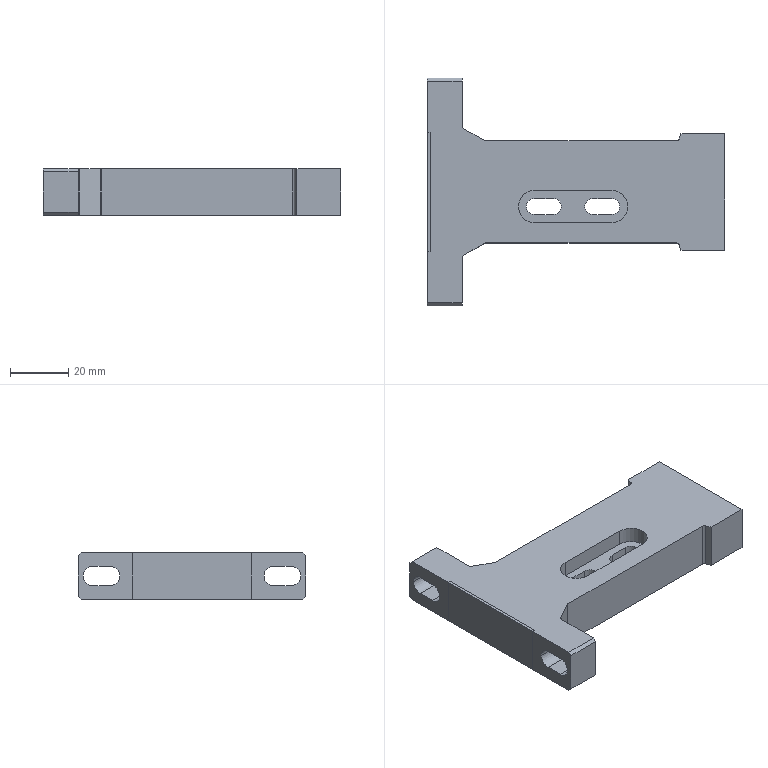NC program | NX | posted with a generic post | part box 102 x 78 x 16 mm
Lines 1 to 852 of 2996:
N10 G17 G21 G94 G90
(ZLEVEL_PROFILE_COPY_COPY_1_COPY_1_COPY_COPY , TOOL : D4)
N12 T04 M6
N14 G54
N16 G17 G0 G90 X-27.95 Y-1.3 B0. C0. S9500 M3
N18 G43 Z30. H4
N20 Z1.5
N22 G94 G1 X-27.838 Z1.494 F1400.
N24 X-27.571 Y-1.238 Z1.48
N26 X-27.322 Y-1.121 Z1.465
N28 X-27.068 Y-0.92 Z1.448
N30 X-26.814 Y-0.556 Z1.425
N32 X-26.696 Y-0.127 Z1.402
N34 X-26.729 Y0.316 Z1.379
N36 X-26.908 Y0.723 Z1.355
N38 X-27.212 Y1.047 Z1.332
N40 X-27.492 Y1.208 Z1.315
N42 X-27.838 Y1.3 Z1.296
N44 X-34.162 Z0.965
N46 X-34.574 Y1.177 Z0.942
N48 X-34.925 Y0.928 Z0.92
N50 X-35.176 Y0.578 Z0.897
N52 X-35.3 Y0.165 Z0.875
N54 Y-0.158 Z0.858
N56 X-35.178 Y-0.573 Z0.835
N58 X-34.928 Y-0.925 Z0.812
N60 X-34.576 Y-1.177 Z0.79
N62 X-34.162 Y-1.3 Z0.767
N64 X-27.838 Z0.436
N66 X-27.571 Y-1.238 Z0.421
N68 X-27.322 Y-1.121 Z0.407
N70 X-27.068 Y-0.92 Z0.39
N72 X-26.814 Y-0.556 Z0.367
N74 X-26.696 Y-0.127 Z0.343
N76 X-26.729 Y0.316 Z0.32
N78 X-26.908 Y0.723 Z0.297
N80 X-27.212 Y1.047 Z0.273
N82 X-27.492 Y1.208 Z0.256
N84 X-27.838 Y1.3 Z0.238
N86 X-34.162 Z-0.094
N88 X-34.574 Y1.177 Z-0.116
N90 X-34.925 Y0.928 Z-0.139
N92 X-35.176 Y0.578 Z-0.161
N94 X-35.3 Y0.165 Z-0.184
N96 Y-0.158 Z-0.201
N98 X-35.178 Y-0.573 Z-0.224
N100 X-34.928 Y-0.925 Z-0.246
N102 X-34.576 Y-1.177 Z-0.269
N104 X-34.162 Y-1.3 Z-0.292
N106 X-34. Z-0.3
N108 X-28.
N110 G3 X-26.7 Y0. R1.3
N112 X-28. Y1.3 R1.3
N114 G1 X-34.
N116 G3 X-35.3 Y0. R1.3
N118 X-34. Y-1.3 R1.3
N120 G1 X-28.118 Z-0.417
N122 X-27.978 Y-1.294 Z-0.419
N124 X-27.839 Y-1.284 Z-0.422
N126 X-27.686 Y-1.254 Z-0.425
N128 X-27.568 Y-1.219 Z-0.428
N130 X-27.422 Y-1.158 Z-0.431
N132 X-27.318 Y-1.098 Z-0.433
N134 X-27.179 Y-0.997 Z-0.437
N136 X-27.098 Y-0.928 Z-0.439
N138 X-26.998 Y-0.821 Z-0.442
N140 X-26.922 Y-0.712 Z-0.444
N142 X-26.832 Y-0.553 Z-0.448
N144 X-26.792 Y-0.467 Z-0.45
N146 X-26.752 Y-0.337 Z-0.453
N148 X-26.723 Y-0.197 Z-0.456
N150 X-26.702 Y-0.077 Z-0.458
N152 X-26.703 Y0.081 Z-0.461
N154 X-26.75 Y0.357 Z-0.467
N156 X-26.798 Y0.496 Z-0.47
N158 X-26.855 Y0.616 Z-0.472
N160 X-26.936 Y0.733 Z-0.475
N162 X-27.018 Y0.842 Z-0.478
N164 X-27.088 Y0.918 Z-0.48
N166 X-27.125 Y0.955 Z-0.481
N168 X-27.221 Y1.032 Z-0.483
N170 X-27.368 Y1.127 Z-0.487
N172 X-27.459 Y1.176 Z-0.489
N174 X-27.596 Y1.229 Z-0.492
N176 X-27.724 Y1.262 Z-0.494
N178 X-27.861 Y1.286 Z-0.497
N180 X-28. Y1.295 Z-0.5
N182 X-28.14 Y1.3 Z-0.503
N184 X-33.042 Z-0.6
N186 X-34.
N188 G3 X-35.3 Y0. R1.3
N190 X-34. Y-1.3 R1.3
N192 G1 X-28.118 Z-0.717
N194 X-27.978 Y-1.294 Z-0.719
N196 X-27.839 Y-1.284 Z-0.722
N198 X-27.686 Y-1.254 Z-0.725
N200 X-27.568 Y-1.219 Z-0.728
N202 X-27.422 Y-1.158 Z-0.731
N204 X-27.318 Y-1.098 Z-0.733
N206 X-27.179 Y-0.997 Z-0.737
N208 X-27.098 Y-0.928 Z-0.739
N210 X-26.998 Y-0.821 Z-0.742
N212 X-26.922 Y-0.712 Z-0.744
N214 X-26.832 Y-0.553 Z-0.748
N216 X-26.792 Y-0.467 Z-0.75
N218 X-26.752 Y-0.337 Z-0.753
N220 X-26.723 Y-0.197 Z-0.756
N222 X-26.702 Y-0.077 Z-0.758
N224 X-26.703 Y0.081 Z-0.761
N226 X-26.75 Y0.357 Z-0.767
N228 X-26.798 Y0.496 Z-0.77
N230 X-26.855 Y0.616 Z-0.772
N232 X-26.936 Y0.733 Z-0.775
N234 X-27.018 Y0.842 Z-0.778
N236 X-27.089 Y0.918 Z-0.78
N238 X-27.125 Y0.955 Z-0.781
N240 X-27.221 Y1.032 Z-0.783
N242 X-27.368 Y1.127 Z-0.787
N244 X-27.459 Y1.176 Z-0.789
N246 X-27.596 Y1.229 Z-0.792
N248 X-27.724 Y1.262 Z-0.794
N250 X-27.861 Y1.286 Z-0.797
N252 X-28. Y1.295 Z-0.8
N254 X-28.14 Y1.3 Z-0.803
N256 X-33.042 Z-0.9
N258 X-34.
N260 G3 X-35.3 Y0. R1.3
N262 X-34. Y-1.3 R1.3
N264 G1 X-28.118 Z-1.017
N266 X-27.978 Y-1.294 Z-1.019
N268 X-27.839 Y-1.284 Z-1.022
N270 X-27.686 Y-1.254 Z-1.025
N272 X-27.568 Y-1.219 Z-1.028
N274 X-27.422 Y-1.158 Z-1.031
N276 X-27.318 Y-1.098 Z-1.033
N278 X-27.179 Y-0.997 Z-1.037
N280 X-27.098 Y-0.928 Z-1.039
N282 X-26.998 Y-0.821 Z-1.042
N284 X-26.922 Y-0.712 Z-1.044
N286 X-26.832 Y-0.553 Z-1.048
N288 X-26.792 Y-0.467 Z-1.05
N290 X-26.752 Y-0.337 Z-1.053
N292 X-26.723 Y-0.197 Z-1.056
N294 X-26.702 Y-0.077 Z-1.058
N296 X-26.703 Y0.081 Z-1.061
N298 X-26.75 Y0.357 Z-1.067
N300 X-26.798 Y0.496 Z-1.07
N302 X-26.855 Y0.616 Z-1.072
N304 X-26.936 Y0.733 Z-1.075
N306 X-27.018 Y0.842 Z-1.078
N308 X-27.089 Y0.918 Z-1.08
N310 X-27.125 Y0.955 Z-1.081
N312 X-27.221 Y1.032 Z-1.083
N314 X-27.368 Y1.127 Z-1.087
N316 X-27.459 Y1.176 Z-1.089
N318 X-27.596 Y1.229 Z-1.092
N320 X-27.724 Y1.262 Z-1.094
N322 X-27.861 Y1.285 Z-1.097
N324 X-28. Y1.295 Z-1.1
N326 X-28.14 Y1.3 Z-1.103
N328 X-33.042 Z-1.2
N330 X-34.
N332 G3 X-35.3 Y0. R1.3
N334 X-34. Y-1.3 R1.3
N336 G1 X-28.118 Z-1.317
N338 X-27.978 Y-1.294 Z-1.319
N340 X-27.839 Y-1.284 Z-1.322
N342 X-27.686 Y-1.254 Z-1.325
N344 X-27.568 Y-1.219 Z-1.328
N346 X-27.422 Y-1.158 Z-1.331
N348 X-27.318 Y-1.098 Z-1.333
N350 X-27.179 Y-0.997 Z-1.337
N352 X-27.098 Y-0.928 Z-1.339
N354 X-26.998 Y-0.821 Z-1.342
N356 X-26.922 Y-0.712 Z-1.344
N358 X-26.832 Y-0.553 Z-1.348
N360 X-26.792 Y-0.467 Z-1.35
N362 X-26.752 Y-0.337 Z-1.353
N364 X-26.723 Y-0.197 Z-1.356
N366 X-26.702 Y-0.077 Z-1.358
N368 X-26.703 Y0.081 Z-1.361
N370 X-26.75 Y0.357 Z-1.367
N372 X-26.798 Y0.496 Z-1.37
N374 X-26.855 Y0.616 Z-1.372
N376 X-26.936 Y0.733 Z-1.375
N378 X-27.018 Y0.842 Z-1.378
N380 X-27.089 Y0.918 Z-1.38
N382 X-27.125 Y0.955 Z-1.381
N384 X-27.221 Y1.032 Z-1.383
N386 X-27.368 Y1.127 Z-1.387
N388 X-27.459 Y1.176 Z-1.389
N390 X-27.596 Y1.229 Z-1.392
N392 X-27.724 Y1.262 Z-1.394
N394 X-27.861 Y1.285 Z-1.397
N396 X-28. Y1.295 Z-1.4
N398 X-28.14 Y1.3 Z-1.403
N400 X-33.042 Z-1.5
N402 X-34.
N404 G3 X-35.3 Y0. R1.3
N406 X-34. Y-1.3 R1.3
N408 G1 X-28.118 Z-1.617
N410 X-27.978 Y-1.294 Z-1.619
N412 X-27.839 Y-1.284 Z-1.622
N414 X-27.686 Y-1.254 Z-1.625
N416 X-27.568 Y-1.219 Z-1.628
N418 X-27.422 Y-1.158 Z-1.631
N420 X-27.318 Y-1.098 Z-1.633
N422 X-27.179 Y-0.997 Z-1.637
N424 X-27.098 Y-0.928 Z-1.639
N426 X-26.998 Y-0.821 Z-1.642
N428 X-26.922 Y-0.712 Z-1.644
N430 X-26.832 Y-0.553 Z-1.648
N432 X-26.792 Y-0.467 Z-1.65
N434 X-26.752 Y-0.337 Z-1.653
N436 X-26.723 Y-0.197 Z-1.656
N438 X-26.702 Y-0.077 Z-1.658
N440 X-26.703 Y0.081 Z-1.661
N442 X-26.75 Y0.357 Z-1.667
N444 X-26.798 Y0.496 Z-1.67
N446 X-26.855 Y0.616 Z-1.672
N448 X-26.936 Y0.733 Z-1.675
N450 X-27.018 Y0.842 Z-1.678
N452 X-27.089 Y0.918 Z-1.68
N454 X-27.125 Y0.955 Z-1.681
N456 X-27.221 Y1.032 Z-1.683
N458 X-27.368 Y1.127 Z-1.687
N460 X-27.459 Y1.176 Z-1.689
N462 X-27.595 Y1.229 Z-1.692
N464 X-27.724 Y1.262 Z-1.694
N466 X-27.861 Y1.285 Z-1.697
N468 X-28. Y1.295 Z-1.7
N470 X-28.14 Y1.3 Z-1.703
N472 X-33.042 Z-1.8
N474 X-34.
N476 G3 X-35.3 Y0. R1.3
N478 X-34. Y-1.3 R1.3
N480 G1 X-28.118 Z-1.917
N482 X-27.978 Y-1.294 Z-1.919
N484 X-27.839 Y-1.284 Z-1.922
N486 X-27.686 Y-1.254 Z-1.925
N488 X-27.568 Y-1.219 Z-1.928
N490 X-27.422 Y-1.158 Z-1.931
N492 X-27.318 Y-1.098 Z-1.933
N494 X-27.179 Y-0.997 Z-1.937
N496 X-27.098 Y-0.928 Z-1.939
N498 X-26.999 Y-0.821 Z-1.942
N500 X-26.922 Y-0.712 Z-1.944
N502 X-26.832 Y-0.553 Z-1.948
N504 X-26.792 Y-0.467 Z-1.95
N506 X-26.752 Y-0.337 Z-1.953
N508 X-26.723 Y-0.197 Z-1.956
N510 X-26.702 Y-0.077 Z-1.958
N512 X-26.703 Y0.081 Z-1.961
N514 X-26.75 Y0.357 Z-1.967
N516 X-26.798 Y0.496 Z-1.97
N518 X-26.855 Y0.616 Z-1.972
N520 X-26.936 Y0.733 Z-1.975
N522 X-27.018 Y0.842 Z-1.978
N524 X-27.089 Y0.918 Z-1.98
N526 X-27.125 Y0.955 Z-1.981
N528 X-27.221 Y1.032 Z-1.983
N530 X-27.368 Y1.127 Z-1.987
N532 X-27.459 Y1.176 Z-1.989
N534 X-27.595 Y1.229 Z-1.992
N536 X-27.724 Y1.262 Z-1.994
N538 X-27.861 Y1.285 Z-1.997
N540 X-28. Y1.295 Z-2.
N542 X-28.14 Y1.3 Z-2.003
N544 X-33.042 Z-2.1
N546 X-34.
N548 G3 X-35.3 Y0. R1.3
N550 X-34. Y-1.3 R1.3
N552 G1 X-28.118 Z-2.217
N554 X-27.978 Y-1.294 Z-2.219
N556 X-27.839 Y-1.284 Z-2.222
N558 X-27.686 Y-1.254 Z-2.225
N560 X-27.568 Y-1.219 Z-2.228
N562 X-27.422 Y-1.158 Z-2.231
N564 X-27.318 Y-1.098 Z-2.233
N566 X-27.179 Y-0.997 Z-2.237
N568 X-27.098 Y-0.928 Z-2.239
N570 X-26.999 Y-0.821 Z-2.242
N572 X-26.922 Y-0.712 Z-2.244
N574 X-26.832 Y-0.553 Z-2.248
N576 X-26.792 Y-0.467 Z-2.25
N578 X-26.752 Y-0.337 Z-2.253
N580 X-26.723 Y-0.197 Z-2.256
N582 X-26.702 Y-0.077 Z-2.258
N584 X-26.703 Y0.081 Z-2.261
N586 X-26.75 Y0.357 Z-2.267
N588 X-26.798 Y0.496 Z-2.27
N590 X-26.855 Y0.616 Z-2.272
N592 X-26.936 Y0.733 Z-2.275
N594 X-27.018 Y0.842 Z-2.278
N596 X-27.089 Y0.918 Z-2.28
N598 X-27.125 Y0.955 Z-2.281
N600 X-27.221 Y1.032 Z-2.283
N602 X-27.368 Y1.127 Z-2.287
N604 X-27.459 Y1.176 Z-2.289
N606 X-27.595 Y1.229 Z-2.292
N608 X-27.724 Y1.262 Z-2.294
N610 X-27.861 Y1.285 Z-2.297
N612 X-28. Y1.295 Z-2.3
N614 X-28.14 Y1.3 Z-2.303
N616 X-33.042 Z-2.4
N618 X-34.
N620 G3 X-35.3 Y0. R1.3
N622 X-34. Y-1.3 R1.3
N624 G1 X-28.118 Z-2.517
N626 X-27.978 Y-1.294 Z-2.519
N628 X-27.839 Y-1.284 Z-2.522
N630 X-27.686 Y-1.254 Z-2.525
N632 X-27.568 Y-1.219 Z-2.528
N634 X-27.422 Y-1.158 Z-2.531
N636 X-27.318 Y-1.098 Z-2.533
N638 X-27.179 Y-0.997 Z-2.537
N640 X-27.098 Y-0.928 Z-2.539
N642 X-26.999 Y-0.821 Z-2.542
N644 X-26.922 Y-0.712 Z-2.544
N646 X-26.832 Y-0.553 Z-2.548
N648 X-26.792 Y-0.467 Z-2.55
N650 X-26.752 Y-0.337 Z-2.553
N652 X-26.723 Y-0.197 Z-2.556
N654 X-26.702 Y-0.077 Z-2.558
N656 X-26.703 Y0.081 Z-2.561
N658 X-26.75 Y0.357 Z-2.567
N660 X-26.798 Y0.496 Z-2.57
N662 X-26.855 Y0.616 Z-2.572
N664 X-26.936 Y0.733 Z-2.575
N666 X-27.018 Y0.842 Z-2.578
N668 X-27.089 Y0.918 Z-2.58
N670 X-27.125 Y0.955 Z-2.581
N672 X-27.221 Y1.032 Z-2.583
N674 X-27.368 Y1.127 Z-2.587
N676 X-27.459 Y1.176 Z-2.589
N678 X-27.595 Y1.229 Z-2.592
N680 X-27.724 Y1.262 Z-2.594
N682 X-27.861 Y1.285 Z-2.597
N684 X-28. Y1.295 Z-2.6
N686 X-28.14 Y1.3 Z-2.603
N688 X-33.042 Z-2.7
N690 X-34.
N692 G3 X-35.3 Y0. R1.3
N694 X-34. Y-1.3 R1.3
N696 G1 X-28.118 Z-2.817
N698 X-27.978 Y-1.294 Z-2.819
N700 X-27.839 Y-1.284 Z-2.822
N702 X-27.686 Y-1.254 Z-2.825
N704 X-27.568 Y-1.219 Z-2.828
N706 X-27.422 Y-1.158 Z-2.831
N708 X-27.318 Y-1.098 Z-2.833
N710 X-27.179 Y-0.997 Z-2.837
N712 X-27.098 Y-0.928 Z-2.839
N714 X-26.999 Y-0.821 Z-2.842
N716 X-26.922 Y-0.712 Z-2.844
N718 X-26.832 Y-0.553 Z-2.848
N720 X-26.792 Y-0.467 Z-2.85
N722 X-26.752 Y-0.337 Z-2.853
N724 X-26.723 Y-0.197 Z-2.856
N726 X-26.702 Y-0.077 Z-2.858
N728 X-26.703 Y0.081 Z-2.861
N730 X-26.75 Y0.357 Z-2.867
N732 X-26.798 Y0.496 Z-2.87
N734 X-26.855 Y0.616 Z-2.872
N736 X-26.936 Y0.733 Z-2.875
N738 X-27.018 Y0.842 Z-2.878
N740 X-27.089 Y0.918 Z-2.88
N742 X-27.125 Y0.955 Z-2.881
N744 X-27.221 Y1.032 Z-2.883
N746 X-27.368 Y1.127 Z-2.887
N748 X-27.459 Y1.176 Z-2.889
N750 X-27.595 Y1.229 Z-2.892
N752 X-27.724 Y1.262 Z-2.894
N754 X-27.861 Y1.285 Z-2.897
N756 X-28. Y1.295 Z-2.9
N758 X-28.14 Y1.3 Z-2.903
N760 X-33.042 Z-3.
N762 X-34.
N764 G3 X-35.3 Y0. R1.3
N766 X-34. Y-1.3 R1.3
N768 G1 X-28.118 Z-3.117
N770 X-27.978 Y-1.294 Z-3.119
N772 X-27.839 Y-1.284 Z-3.122
N774 X-27.686 Y-1.254 Z-3.125
N776 X-27.568 Y-1.219 Z-3.128
N778 X-27.422 Y-1.158 Z-3.131
N780 X-27.318 Y-1.098 Z-3.133
N782 X-27.179 Y-0.997 Z-3.137
N784 X-27.098 Y-0.928 Z-3.139
N786 X-26.999 Y-0.821 Z-3.142
N788 X-26.922 Y-0.712 Z-3.144
N790 X-26.832 Y-0.553 Z-3.148
N792 X-26.792 Y-0.467 Z-3.15
N794 X-26.752 Y-0.337 Z-3.153
N796 X-26.723 Y-0.197 Z-3.156
N798 X-26.702 Y-0.077 Z-3.158
N800 X-26.703 Y0.081 Z-3.161
N802 X-26.75 Y0.357 Z-3.167
N804 X-26.798 Y0.496 Z-3.17
N806 X-26.855 Y0.616 Z-3.172
N808 X-26.936 Y0.733 Z-3.175
N810 X-27.018 Y0.842 Z-3.178
N812 X-27.089 Y0.918 Z-3.18
N814 X-27.125 Y0.955 Z-3.181
N816 X-27.221 Y1.032 Z-3.183
N818 X-27.368 Y1.127 Z-3.187
N820 X-27.459 Y1.176 Z-3.189
N822 X-27.595 Y1.229 Z-3.192
N824 X-27.724 Y1.262 Z-3.194
N826 X-27.861 Y1.285 Z-3.197
N828 X-28. Y1.295 Z-3.2
N830 X-28.14 Y1.3 Z-3.203
N832 X-33.042 Z-3.3
N834 X-34.
N836 G3 X-35.3 Y0. R1.3
N838 X-34. Y-1.3 R1.3
N840 G1 X-28.118 Z-3.417
N842 X-27.978 Y-1.294 Z-3.419
N844 X-27.839 Y-1.284 Z-3.422
N846 X-27.686 Y-1.254 Z-3.425
N848 X-27.568 Y-1.219 Z-3.428
N850 X-27.422 Y-1.158 Z-3.431
N852 X-27.318 Y-1.098 Z-3.433
N854 X-27.179 Y-0.997 Z-3.437
N856 X-27.098 Y-0.928 Z-3.439
N858 X-26.999 Y-0.821 Z-3.442
N860 X-26.922 Y-0.712 Z-3.444
N862 X-26.832 Y-0.553 Z-3.448
N864 X-26.792 Y-0.467 Z-3.45
N866 X-26.752 Y-0.337 Z-3.453
N868 X-26.723 Y-0.197 Z-3.456
N870 X-26.702 Y-0.077 Z-3.458
N872 X-26.703 Y0.081 Z-3.461
N874 X-26.75 Y0.357 Z-3.467
N876 X-26.798 Y0.496 Z-3.47
N878 X-26.855 Y0.616 Z-3.472
N880 X-26.936 Y0.733 Z-3.475
N882 X-27.018 Y0.842 Z-3.478
N884 X-27.089 Y0.918 Z-3.48
N886 X-27.125 Y0.955 Z-3.481
N888 X-27.221 Y1.032 Z-3.483
N890 X-27.368 Y1.127 Z-3.487
N892 X-27.459 Y1.176 Z-3.489
N894 X-27.595 Y1.229 Z-3.492
N896 X-27.724 Y1.262 Z-3.494
N898 X-27.861 Y1.285 Z-3.497
N900 X-28. Y1.295 Z-3.5
N902 X-28.14 Y1.3 Z-3.503
N904 X-33.042 Z-3.6
N906 X-34.
N908 G3 X-35.3 Y0. R1.3
N910 X-34. Y-1.3 R1.3
N912 G1 X-28.118 Z-3.717
N914 X-27.978 Y-1.294 Z-3.719
N916 X-27.839 Y-1.284 Z-3.722
N918 X-27.686 Y-1.254 Z-3.725
N920 X-27.568 Y-1.219 Z-3.728
N922 X-27.422 Y-1.158 Z-3.731
N924 X-27.318 Y-1.098 Z-3.733
N926 X-27.179 Y-0.997 Z-3.737
N928 X-27.098 Y-0.928 Z-3.739
N930 X-26.999 Y-0.821 Z-3.742
N932 X-26.922 Y-0.712 Z-3.744
N934 X-26.832 Y-0.553 Z-3.748
N936 X-26.792 Y-0.467 Z-3.75
N938 X-26.752 Y-0.337 Z-3.753
N940 X-26.723 Y-0.197 Z-3.756
N942 X-26.702 Y-0.077 Z-3.758
N944 X-26.703 Y0.081 Z-3.761
N946 X-26.75 Y0.357 Z-3.767
N948 X-26.798 Y0.496 Z-3.77
N950 X-26.855 Y0.616 Z-3.772
N952 X-26.936 Y0.733 Z-3.775
N954 X-27.018 Y0.842 Z-3.778
N956 X-27.089 Y0.918 Z-3.78
N958 X-27.125 Y0.955 Z-3.781
N960 X-27.221 Y1.032 Z-3.783
N962 X-27.368 Y1.127 Z-3.787
N964 X-27.459 Y1.176 Z-3.789
N966 X-27.595 Y1.229 Z-3.792
N968 X-27.724 Y1.262 Z-3.794
N970 X-27.861 Y1.285 Z-3.797
N972 X-28. Y1.295 Z-3.8
N974 X-28.14 Y1.3 Z-3.803
N976 X-33.042 Z-3.9
N978 X-34.
N980 G3 X-35.3 Y0. R1.3
N982 X-34. Y-1.3 R1.3
N984 G1 X-28.118 Z-4.017
N986 X-27.978 Y-1.294 Z-4.019
N988 X-27.839 Y-1.284 Z-4.022
N990 X-27.686 Y-1.254 Z-4.025
N992 X-27.568 Y-1.219 Z-4.028
N994 X-27.422 Y-1.158 Z-4.031
N996 X-27.318 Y-1.098 Z-4.033
N998 X-27.179 Y-0.997 Z-4.037
N1000 X-27.098 Y-0.928 Z-4.039
N1002 X-26.999 Y-0.821 Z-4.042
N1004 X-26.922 Y-0.712 Z-4.044
N1006 X-26.832 Y-0.553 Z-4.048
N1008 X-26.792 Y-0.467 Z-4.05
N1010 X-26.752 Y-0.337 Z-4.053
N1012 X-26.723 Y-0.197 Z-4.056
N1014 X-26.702 Y-0.077 Z-4.058
N1016 X-26.703 Y0.081 Z-4.061
N1018 X-26.75 Y0.357 Z-4.067
N1020 X-26.798 Y0.496 Z-4.07
N1022 X-26.855 Y0.616 Z-4.072
N1024 X-26.936 Y0.733 Z-4.075
N1026 X-27.018 Y0.842 Z-4.078
N1028 X-27.089 Y0.918 Z-4.08
N1030 X-27.125 Y0.955 Z-4.081
N1032 X-27.221 Y1.032 Z-4.083
N1034 X-27.368 Y1.127 Z-4.087
N1036 X-27.459 Y1.176 Z-4.089
N1038 X-27.595 Y1.229 Z-4.092
N1040 X-27.724 Y1.262 Z-4.094
N1042 X-27.861 Y1.285 Z-4.097
N1044 X-28. Y1.295 Z-4.1
N1046 X-28.14 Y1.3 Z-4.103
N1048 X-33.042 Z-4.2
N1050 X-34.
N1052 G3 X-35.3 Y0. R1.3
N1054 X-34. Y-1.3 R1.3
N1056 G1 X-28.118 Z-4.317
N1058 X-27.978 Y-1.294 Z-4.319
N1060 X-27.839 Y-1.284 Z-4.322
N1062 X-27.686 Y-1.254 Z-4.325
N1064 X-27.568 Y-1.219 Z-4.328
N1066 X-27.422 Y-1.158 Z-4.331
N1068 X-27.318 Y-1.098 Z-4.333
N1070 X-27.179 Y-0.997 Z-4.337
N1072 X-27.098 Y-0.928 Z-4.339
N1074 X-26.999 Y-0.821 Z-4.342
N1076 X-26.922 Y-0.712 Z-4.344
N1078 X-26.832 Y-0.553 Z-4.348
N1080 X-26.792 Y-0.467 Z-4.35
N1082 X-26.752 Y-0.337 Z-4.353
N1084 X-26.723 Y-0.197 Z-4.356
N1086 X-26.702 Y-0.077 Z-4.358
N1088 X-26.703 Y0.081 Z-4.361
N1090 X-26.75 Y0.357 Z-4.367
N1092 X-26.798 Y0.496 Z-4.37
N1094 X-26.855 Y0.616 Z-4.372
N1096 X-26.936 Y0.733 Z-4.375
N1098 X-27.018 Y0.842 Z-4.378
N1100 X-27.089 Y0.918 Z-4.38
N1102 X-27.125 Y0.955 Z-4.381
N1104 X-27.221 Y1.032 Z-4.383
N1106 X-27.368 Y1.127 Z-4.387
N1108 X-27.459 Y1.176 Z-4.389
N1110 X-27.595 Y1.229 Z-4.392
N1112 X-27.724 Y1.262 Z-4.394
N1114 X-27.861 Y1.285 Z-4.397
N1116 X-28. Y1.295 Z-4.4
N1118 X-28.14 Y1.3 Z-4.403
N1120 X-33.042 Z-4.5
N1122 X-34.
N1124 G3 X-35.3 Y0. R1.3
N1126 X-34. Y-1.3 R1.3
N1128 G1 X-28.118 Z-4.617
N1130 X-27.978 Y-1.294 Z-4.619
N1132 X-27.839 Y-1.284 Z-4.622
N1134 X-27.686 Y-1.254 Z-4.625
N1136 X-27.568 Y-1.219 Z-4.628
N1138 X-27.422 Y-1.158 Z-4.631
N1140 X-27.318 Y-1.098 Z-4.633
N1142 X-27.179 Y-0.997 Z-4.637
N1144 X-27.098 Y-0.928 Z-4.639
N1146 X-26.999 Y-0.821 Z-4.642
N1148 X-26.922 Y-0.712 Z-4.644
N1150 X-26.832 Y-0.553 Z-4.648
N1152 X-26.792 Y-0.467 Z-4.65
N1154 X-26.752 Y-0.337 Z-4.653
N1156 X-26.723 Y-0.197 Z-4.656
N1158 X-26.702 Y-0.077 Z-4.658
N1160 X-26.703 Y0.081 Z-4.661
N1162 X-26.75 Y0.357 Z-4.667
N1164 X-26.798 Y0.496 Z-4.67
N1166 X-26.855 Y0.616 Z-4.672
N1168 X-26.936 Y0.733 Z-4.675
N1170 X-27.018 Y0.842 Z-4.678
N1172 X-27.125 Y0.955 Z-4.681
N1174 X-27.221 Y1.032 Z-4.683
N1176 X-27.368 Y1.127 Z-4.687
N1178 X-27.459 Y1.176 Z-4.689
N1180 X-27.595 Y1.229 Z-4.692
N1182 X-27.724 Y1.262 Z-4.694
N1184 X-27.861 Y1.285 Z-4.697
N1186 X-28. Y1.295 Z-4.7
N1188 X-28.14 Y1.3 Z-4.703
N1190 X-33.042 Z-4.8
N1192 X-34.
N1194 G3 X-35.3 Y0. R1.3
N1196 X-34. Y-1.3 R1.3
N1198 G1 X-28.118 Z-4.917
N1200 X-27.978 Y-1.294 Z-4.919
N1202 X-27.839 Y-1.284 Z-4.922
N1204 X-27.686 Y-1.254 Z-4.925
N1206 X-27.568 Y-1.219 Z-4.928
N1208 X-27.422 Y-1.158 Z-4.931
N1210 X-27.318 Y-1.098 Z-4.933
N1212 X-27.179 Y-0.997 Z-4.937
N1214 X-27.098 Y-0.928 Z-4.939
N1216 X-26.999 Y-0.821 Z-4.942
N1218 X-26.922 Y-0.712 Z-4.944
N1220 X-26.832 Y-0.553 Z-4.948
N1222 X-26.792 Y-0.467 Z-4.95
N1224 X-26.752 Y-0.337 Z-4.953
N1226 X-26.723 Y-0.197 Z-4.956
N1228 X-26.702 Y-0.077 Z-4.958
N1230 X-26.703 Y0.081 Z-4.961
N1232 X-26.75 Y0.357 Z-4.967
N1234 X-26.798 Y0.496 Z-4.97
N1236 X-26.855 Y0.616 Z-4.972
N1238 X-26.936 Y0.733 Z-4.975
N1240 X-27.018 Y0.842 Z-4.978
N1242 X-27.125 Y0.955 Z-4.981
N1244 X-27.221 Y1.032 Z-4.983
N1246 X-27.368 Y1.127 Z-4.987
N1248 X-27.459 Y1.176 Z-4.989
N1250 X-27.595 Y1.229 Z-4.992
N1252 X-27.724 Y1.262 Z-4.994
N1254 X-27.861 Y1.285 Z-4.997
N1256 X-28. Y1.295 Z-5.
N1258 X-28.14 Y1.3 Z-5.003
N1260 X-33.042 Z-5.1
N1262 X-34.
N1264 G3 X-35.3 Y0. R1.3
N1266 X-34. Y-1.3 R1.3
N1268 G1 X-28.118 Z-5.217
N1270 X-27.978 Y-1.294 Z-5.219
N1272 X-27.839 Y-1.284 Z-5.222
N1274 X-27.686 Y-1.254 Z-5.225
N1276 X-27.568 Y-1.219 Z-5.228
N1278 X-27.422 Y-1.158 Z-5.231
N1280 X-27.318 Y-1.098 Z-5.233
N1282 X-27.179 Y-0.997 Z-5.237
N1284 X-27.098 Y-0.928 Z-5.239
N1286 X-26.999 Y-0.821 Z-5.242
N1288 X-26.922 Y-0.712 Z-5.244
N1290 X-26.832 Y-0.553 Z-5.248
N1292 X-26.792 Y-0.467 Z-5.25
N1294 X-26.752 Y-0.337 Z-5.253
N1296 X-26.723 Y-0.197 Z-5.256
N1298 X-26.702 Y-0.077 Z-5.258
N1300 X-26.703 Y0.081 Z-5.261
N1302 X-26.75 Y0.357 Z-5.267
N1304 X-26.798 Y0.496 Z-5.27
N1306 X-26.855 Y0.616 Z-5.272
N1308 X-26.936 Y0.733 Z-5.275
N1310 X-27.018 Y0.842 Z-5.278
N1312 X-27.125 Y0.955 Z-5.281
N1314 X-27.221 Y1.032 Z-5.283
N1316 X-27.368 Y1.127 Z-5.287
N1318 X-27.459 Y1.176 Z-5.289
N1320 X-27.595 Y1.229 Z-5.292
N1322 X-27.724 Y1.262 Z-5.294
N1324 X-27.861 Y1.285 Z-5.297
N1326 X-28. Y1.295 Z-5.3
N1328 X-28.14 Y1.3 Z-5.303
N1330 X-33.042 Z-5.4
N1332 X-34.
N1334 G3 X-35.3 Y0. R1.3
N1336 X-34. Y-1.3 R1.3
N1338 G1 X-28.118 Z-5.517
N1340 X-27.978 Y-1.294 Z-5.519
N1342 X-27.839 Y-1.284 Z-5.522
N1344 X-27.686 Y-1.254 Z-5.525
N1346 X-27.568 Y-1.219 Z-5.528
N1348 X-27.422 Y-1.158 Z-5.531
N1350 X-27.318 Y-1.098 Z-5.533
N1352 X-27.179 Y-0.997 Z-5.537
N1354 X-27.098 Y-0.928 Z-5.539
N1356 X-26.999 Y-0.821 Z-5.542
N1358 X-26.922 Y-0.712 Z-5.544
N1360 X-26.832 Y-0.553 Z-5.548
N1362 X-26.792 Y-0.467 Z-5.55
N1364 X-26.752 Y-0.337 Z-5.553
N1366 X-26.723 Y-0.197 Z-5.556
N1368 X-26.702 Y-0.077 Z-5.558
N1370 X-26.703 Y0.081 Z-5.561
N1372 X-26.75 Y0.357 Z-5.567
N1374 X-26.798 Y0.496 Z-5.57
N1376 X-26.855 Y0.616 Z-5.572
N1378 X-26.936 Y0.733 Z-5.575
N1380 X-27.018 Y0.842 Z-5.578
N1382 X-27.125 Y0.955 Z-5.581
N1384 X-27.221 Y1.032 Z-5.583
N1386 X-27.368 Y1.127 Z-5.587
N1388 X-27.459 Y1.176 Z-5.589
N1390 X-27.595 Y1.229 Z-5.592
N1392 X-27.724 Y1.262 Z-5.594
N1394 X-27.861 Y1.285 Z-5.597
N1396 X-28. Y1.295 Z-5.6
N1398 X-28.14 Y1.3 Z-5.603
N1400 X-33.042 Z-5.7
N1402 X-34.
N1404 G3 X-35.3 Y0. R1.3
N1406 X-34. Y-1.3 R1.3
N1408 G1 X-28.118 Z-5.817
N1410 X-27.978 Y-1.294 Z-5.819
N1412 X-27.839 Y-1.284 Z-5.822
N1414 X-27.686 Y-1.254 Z-5.825
N1416 X-27.568 Y-1.219 Z-5.828
N1418 X-27.422 Y-1.158 Z-5.831
N1420 X-27.318 Y-1.098 Z-5.833
N1422 X-27.179 Y-0.997 Z-5.837
N1424 X-27.098 Y-0.928 Z-5.839
N1426 X-26.999 Y-0.821 Z-5.842
N1428 X-26.922 Y-0.712 Z-5.844
N1430 X-26.832 Y-0.553 Z-5.848
N1432 X-26.792 Y-0.467 Z-5.85
N1434 X-26.752 Y-0.337 Z-5.853
N1436 X-26.723 Y-0.197 Z-5.856
N1438 X-26.702 Y-0.077 Z-5.858
N1440 X-26.703 Y0.081 Z-5.861
N1442 X-26.75 Y0.357 Z-5.867
N1444 X-26.798 Y0.496 Z-5.87
N1446 X-26.855 Y0.616 Z-5.872
N1448 X-26.936 Y0.733 Z-5.875
N1450 X-27.018 Y0.842 Z-5.878
N1452 X-27.125 Y0.955 Z-5.881
N1454 X-27.221 Y1.032 Z-5.883
N1456 X-27.368 Y1.127 Z-5.887
N1458 X-27.459 Y1.176 Z-5.889
N1460 X-27.595 Y1.229 Z-5.892
N1462 X-27.724 Y1.262 Z-5.894
N1464 X-27.861 Y1.285 Z-5.897
N1466 X-28. Y1.295 Z-5.9
N1468 X-28.14 Y1.3 Z-5.903
N1470 X-33.042 Z-6.
N1472 X-34.
N1474 G3 X-35.3 Y0. R1.3
N1476 X-34. Y-1.3 R1.3
N1478 G1 X-28.118 Z-6.117
N1480 X-27.978 Y-1.294 Z-6.119
N1482 X-27.839 Y-1.284 Z-6.122
N1484 X-27.686 Y-1.254 Z-6.125
N1486 X-27.568 Y-1.219 Z-6.128
N1488 X-27.422 Y-1.158 Z-6.131
N1490 X-27.318 Y-1.098 Z-6.133
N1492 X-27.179 Y-0.997 Z-6.137
N1494 X-27.098 Y-0.928 Z-6.139
N1496 X-26.999 Y-0.821 Z-6.142
N1498 X-26.922 Y-0.712 Z-6.144
N1500 X-26.832 Y-0.553 Z-6.148
N1502 X-26.792 Y-0.467 Z-6.15
N1504 X-26.752 Y-0.337 Z-6.153
N1506 X-26.723 Y-0.197 Z-6.156
N1508 X-26.702 Y-0.077 Z-6.158
N1510 X-26.703 Y0.081 Z-6.161
N1512 X-26.75 Y0.357 Z-6.167
N1514 X-26.798 Y0.496 Z-6.17
N1516 X-26.855 Y0.616 Z-6.172
N1518 X-26.936 Y0.733 Z-6.175
N1520 X-27.018 Y0.842 Z-6.178
N1522 X-27.125 Y0.955 Z-6.181
N1524 X-27.221 Y1.032 Z-6.183
N1526 X-27.368 Y1.127 Z-6.187
N1528 X-27.459 Y1.176 Z-6.189
N1530 X-27.595 Y1.229 Z-6.192
N1532 X-27.724 Y1.262 Z-6.194
N1534 X-27.861 Y1.285 Z-6.197
N1536 X-28. Y1.295 Z-6.2
N1538 X-28.14 Y1.3 Z-6.203
N1540 X-33.042 Z-6.3
N1542 X-34.
N1544 G3 X-35.3 Y0. R1.3
N1546 X-34. Y-1.3 R1.3
N1548 G1 X-28.118 Z-6.417
N1550 X-27.978 Y-1.294 Z-6.419
N1552 X-27.839 Y-1.284 Z-6.422
N1554 X-27.686 Y-1.254 Z-6.425
N1556 X-27.568 Y-1.219 Z-6.428
N1558 X-27.422 Y-1.158 Z-6.431
N1560 X-27.318 Y-1.098 Z-6.433
N1562 X-27.179 Y-0.997 Z-6.437
N1564 X-27.098 Y-0.928 Z-6.439
N1566 X-26.999 Y-0.821 Z-6.442
N1568 X-26.922 Y-0.712 Z-6.444
N1570 X-26.832 Y-0.553 Z-6.448
N1572 X-26.792 Y-0.467 Z-6.45
N1574 X-26.752 Y-0.337 Z-6.453
N1576 X-26.723 Y-0.197 Z-6.456
N1578 X-26.702 Y-0.077 Z-6.458
N1580 X-26.703 Y0.081 Z-6.461
N1582 X-26.75 Y0.357 Z-6.467
N1584 X-26.798 Y0.496 Z-6.47
N1586 X-26.855 Y0.616 Z-6.472
N1588 X-26.936 Y0.733 Z-6.475
N1590 X-27.018 Y0.842 Z-6.478
N1592 X-27.125 Y0.955 Z-6.481
N1594 X-27.221 Y1.032 Z-6.483
N1596 X-27.368 Y1.127 Z-6.487
N1598 X-27.459 Y1.176 Z-6.489
N1600 X-27.595 Y1.229 Z-6.492
N1602 X-27.724 Y1.262 Z-6.494
N1604 X-27.861 Y1.285 Z-6.497
N1606 X-28. Y1.295 Z-6.5
N1608 X-28.14 Y1.3 Z-6.503
N1610 X-33.042 Z-6.6
N1612 X-34.
N1614 G3 X-35.3 Y0. R1.3
N1616 X-34. Y-1.3 R1.3
N1618 G1 X-28.118 Z-6.717
N1620 X-27.978 Y-1.294 Z-6.719
N1622 X-27.839 Y-1.284 Z-6.722
N1624 X-27.686 Y-1.254 Z-6.725
N1626 X-27.568 Y-1.219 Z-6.728
N1628 X-27.422 Y-1.158 Z-6.731
N1630 X-27.318 Y-1.098 Z-6.733
N1632 X-27.179 Y-0.997 Z-6.737
N1634 X-27.098 Y-0.928 Z-6.739
N1636 X-26.999 Y-0.821 Z-6.742
N1638 X-26.922 Y-0.712 Z-6.744
N1640 X-26.832 Y-0.553 Z-6.748
N1642 X-26.792 Y-0.467 Z-6.75
N1644 X-26.752 Y-0.337 Z-6.753
N1646 X-26.723 Y-0.197 Z-6.756
N1648 X-26.702 Y-0.077 Z-6.758
N1650 X-26.703 Y0.081 Z-6.761
N1652 X-26.75 Y0.357 Z-6.767
N1654 X-26.798 Y0.496 Z-6.77
N1656 X-26.855 Y0.616 Z-6.772
N1658 X-26.936 Y0.733 Z-6.775
N1660 X-27.018 Y0.842 Z-6.778
N1662 X-27.125 Y0.955 Z-6.781
N1664 X-27.221 Y1.032 Z-6.783
N1666 X-27.368 Y1.127 Z-6.787
N1668 X-27.459 Y1.176 Z-6.789
N1670 X-27.595 Y1.229 Z-6.792
N1672 X-27.724 Y1.262 Z-6.794
N1674 X-27.861 Y1.285 Z-6.797
N1676 X-28. Y1.295 Z-6.8
N1678 X-28.14 Y1.3 Z-6.803
N1680 X-33.042 Z-6.9
N1682 X-34.
N1684 G3 X-35.3 Y0. R1.3
N1686 X-34. Y-1.3 R1.3
N1688 G1 X-28.118 Z-7.017
N1690 X-27.978 Y-1.294 Z-7.019
N1692 X-27.839 Y-1.284 Z-7.022
N1694 X-27.686 Y-1.254 Z-7.025
N1696 X-27.568 Y-1.219 Z-7.028
N1698 X-27.422 Y-1.158 Z-7.031
N1700 X-27.318 Y-1.098 Z-7.033
N1702 X-27.179 Y-0.997 Z-7.037